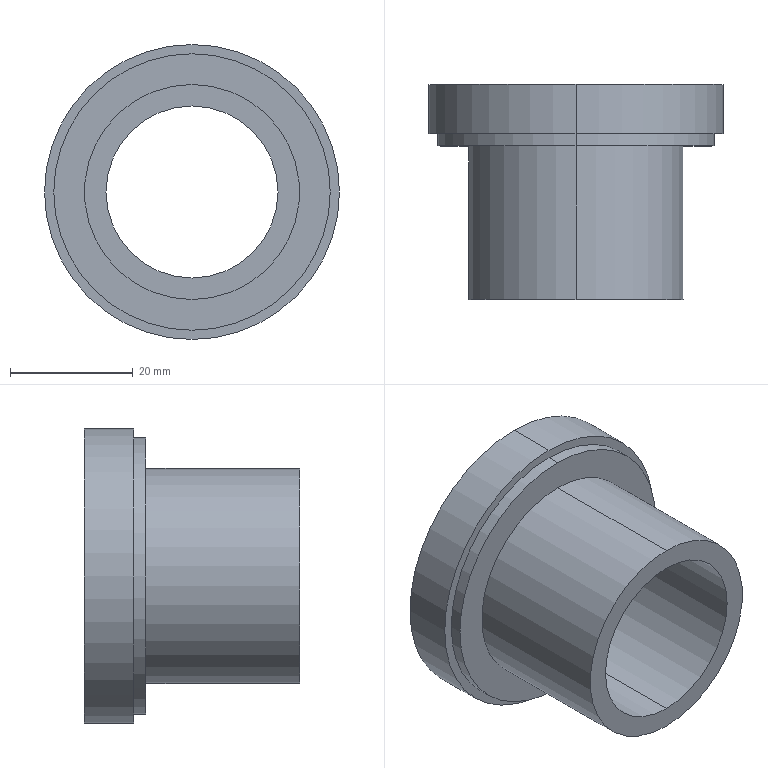Part | SolidWorks | features HoleWzd 1, Revolution 1 | 1 solid | 36 faces | box 48 x 35 x 48 mm | volume 19426 mm3 | cylinder 20 | cone 12 | plane 4 | commonest cylinder face diameters 4.2 x12 28 x2 35 x2 45 x2 48 x2
STEP:
#1=CARTESIAN_POINT('',(-19.,26.6,-2.1));
#2=VERTEX_POINT('',#1);
#3=CARTESIAN_POINT('',(-19.,26.6,2.1));
#4=VERTEX_POINT('',#3);
#5=CARTESIAN_POINT('',(-19.,26.6,0.));
#6=DIRECTION('',(0.,1.,0.));
#7=DIRECTION('',(0.,0.,1.));
#8=AXIS2_PLACEMENT_3D('',#5,#6,#7);
#9=CIRCLE('',#8,2.1);
#10=EDGE_CURVE('',#2,#4,#9,.T.);
#11=ORIENTED_EDGE('',*,*,#10,.F.);
#12=CARTESIAN_POINT('',(-19.,35.,-2.1));
#13=VERTEX_POINT('',#12);
#14=CARTESIAN_POINT('',(-19.,35.,-2.1));
#15=DIRECTION('',(0.,1.,0.));
#16=VECTOR('',#15,1000.);
#17=LINE('',#14,#16);
#18=EDGE_CURVE('',#2,#13,#17,.T.);
#19=ORIENTED_EDGE('',*,*,#18,.T.);
#20=CARTESIAN_POINT('',(-19.,35.,2.1));
#21=VERTEX_POINT('',#20);
#22=CARTESIAN_POINT('',(-19.,35.,0.));
#23=DIRECTION('',(0.,1.,0.));
#24=DIRECTION('',(0.,0.,1.));
#25=AXIS2_PLACEMENT_3D('',#22,#23,#24);
#26=CIRCLE('',#25,2.1);
#27=EDGE_CURVE('',#13,#21,#26,.T.);
#28=ORIENTED_EDGE('',*,*,#27,.T.);
#29=CARTESIAN_POINT('',(-19.,35.,2.1));
#30=DIRECTION('',(0.,1.,0.));
#31=VECTOR('',#30,1000.);
#32=LINE('',#29,#31);
#33=EDGE_CURVE('',#4,#21,#32,.T.);
#34=ORIENTED_EDGE('',*,*,#33,.F.);
#35=EDGE_LOOP('',(#11,#19,#28,#34));
#36=FACE_OUTER_BOUND('',#35,.T.);
#37=CARTESIAN_POINT('',(-19.,35.,0.));
#38=DIRECTION('',(0.,1.,0.));
#39=DIRECTION('',(0.,0.,1.));
#40=AXIS2_PLACEMENT_3D('',#37,#38,#39);
#41=CYLINDRICAL_SURFACE('',#40,2.1);
#42=ADVANCED_FACE('',(#36),#41,.F.);
#43=CARTESIAN_POINT('',(-19.,25.338,0.));
#44=VERTEX_POINT('',#43);
#45=CARTESIAN_POINT('',(-19.,26.6,2.1));
#46=DIRECTION('',(0.,0.515,0.8572));
#47=VECTOR('',#46,1000.);
#48=LINE('',#45,#47);
#49=EDGE_CURVE('',#44,#4,#48,.T.);
#50=ORIENTED_EDGE('',*,*,#49,.F.);
#51=CARTESIAN_POINT('',(-19.,26.6,-2.1));
#52=DIRECTION('',(0.,0.515,-0.8572));
#53=VECTOR('',#52,1000.);
#54=LINE('',#51,#53);
#55=EDGE_CURVE('',#44,#2,#54,.T.);
#56=ORIENTED_EDGE('',*,*,#55,.T.);
#57=ORIENTED_EDGE('',*,*,#10,.T.);
#58=EDGE_LOOP('',(#50,#56,#57));
#59=FACE_OUTER_BOUND('',#58,.T.);
#60=CARTESIAN_POINT('',(-19.,26.6,0.));
#61=DIRECTION('',(0.,1.,0.));
#62=DIRECTION('',(0.,0.,1.));
#63=AXIS2_PLACEMENT_3D('',#60,#61,#62);
#64=CONICAL_SURFACE('',#63,2.1,1.03);
#65=ADVANCED_FACE('',(#59),#64,.F.);
#66=CARTESIAN_POINT('',(19.,26.6,-2.1));
#67=VERTEX_POINT('',#66);
#68=CARTESIAN_POINT('',(19.,26.6,2.1));
#69=VERTEX_POINT('',#68);
#70=CARTESIAN_POINT('',(19.,26.6,0.));
#71=DIRECTION('',(0.,1.,0.));
#72=DIRECTION('',(0.,0.,1.));
#73=AXIS2_PLACEMENT_3D('',#70,#71,#72);
#74=CIRCLE('',#73,2.1);
#75=EDGE_CURVE('',#67,#69,#74,.T.);
#76=ORIENTED_EDGE('',*,*,#75,.F.);
#77=CARTESIAN_POINT('',(19.,35.,-2.1));
#78=VERTEX_POINT('',#77);
#79=CARTESIAN_POINT('',(19.,35.,-2.1));
#80=DIRECTION('',(0.,1.,0.));
#81=VECTOR('',#80,1000.);
#82=LINE('',#79,#81);
#83=EDGE_CURVE('',#67,#78,#82,.T.);
#84=ORIENTED_EDGE('',*,*,#83,.T.);
#85=CARTESIAN_POINT('',(19.,35.,2.1));
#86=VERTEX_POINT('',#85);
#87=CARTESIAN_POINT('',(19.,35.,0.));
#88=DIRECTION('',(0.,1.,0.));
#89=DIRECTION('',(0.,0.,1.));
#90=AXIS2_PLACEMENT_3D('',#87,#88,#89);
#91=CIRCLE('',#90,2.1);
#92=EDGE_CURVE('',#78,#86,#91,.T.);
#93=ORIENTED_EDGE('',*,*,#92,.T.);
#94=CARTESIAN_POINT('',(19.,35.,2.1));
#95=DIRECTION('',(0.,1.,0.));
#96=VECTOR('',#95,1000.);
#97=LINE('',#94,#96);
#98=EDGE_CURVE('',#69,#86,#97,.T.);
#99=ORIENTED_EDGE('',*,*,#98,.F.);
#100=EDGE_LOOP('',(#76,#84,#93,#99));
#101=FACE_OUTER_BOUND('',#100,.T.);
#102=CARTESIAN_POINT('',(19.,35.,0.));
#103=DIRECTION('',(0.,1.,0.));
#104=DIRECTION('',(0.,0.,1.));
#105=AXIS2_PLACEMENT_3D('',#102,#103,#104);
#106=CYLINDRICAL_SURFACE('',#105,2.1);
#107=ADVANCED_FACE('',(#101),#106,.F.);
#108=CARTESIAN_POINT('',(19.,25.338,0.));
#109=VERTEX_POINT('',#108);
#110=CARTESIAN_POINT('',(19.,26.6,2.1));
#111=DIRECTION('',(0.,0.515,0.8572));
#112=VECTOR('',#111,1000.);
#113=LINE('',#110,#112);
#114=EDGE_CURVE('',#109,#69,#113,.T.);
#115=ORIENTED_EDGE('',*,*,#114,.F.);
#116=CARTESIAN_POINT('',(19.,26.6,-2.1));
#117=DIRECTION('',(0.,0.515,-0.8572));
#118=VECTOR('',#117,1000.);
#119=LINE('',#116,#118);
#120=EDGE_CURVE('',#109,#67,#119,.T.);
#121=ORIENTED_EDGE('',*,*,#120,.T.);
#122=ORIENTED_EDGE('',*,*,#75,.T.);
#123=EDGE_LOOP('',(#115,#121,#122));
#124=FACE_OUTER_BOUND('',#123,.T.);
#125=CARTESIAN_POINT('',(19.,26.6,0.));
#126=DIRECTION('',(0.,1.,0.));
#127=DIRECTION('',(0.,0.,1.));
#128=AXIS2_PLACEMENT_3D('',#125,#126,#127);
#129=CONICAL_SURFACE('',#128,2.1,1.03);
#130=ADVANCED_FACE('',(#124),#129,.F.);
#131=CARTESIAN_POINT('',(13.435,26.6,-15.535));
#132=VERTEX_POINT('',#131);
#133=CARTESIAN_POINT('',(13.435,26.6,-11.335));
#134=VERTEX_POINT('',#133);
#135=CARTESIAN_POINT('',(13.435,26.6,-13.435));
#136=DIRECTION('',(0.,1.,0.));
#137=DIRECTION('',(0.,0.,1.));
#138=AXIS2_PLACEMENT_3D('',#135,#136,#137);
#139=CIRCLE('',#138,2.1);
#140=EDGE_CURVE('',#132,#134,#139,.T.);
#141=ORIENTED_EDGE('',*,*,#140,.F.);
#142=CARTESIAN_POINT('',(13.435,35.,-15.535));
#143=VERTEX_POINT('',#142);
#144=CARTESIAN_POINT('',(13.435,35.,-15.535));
#145=DIRECTION('',(0.,1.,0.));
#146=VECTOR('',#145,1000.);
#147=LINE('',#144,#146);
#148=EDGE_CURVE('',#132,#143,#147,.T.);
#149=ORIENTED_EDGE('',*,*,#148,.T.);
#150=CARTESIAN_POINT('',(13.435,35.,-11.335));
#151=VERTEX_POINT('',#150);
#152=CARTESIAN_POINT('',(13.435,35.,-13.435));
#153=DIRECTION('',(0.,1.,0.));
#154=DIRECTION('',(0.,0.,1.));
#155=AXIS2_PLACEMENT_3D('',#152,#153,#154);
#156=CIRCLE('',#155,2.1);
#157=EDGE_CURVE('',#143,#151,#156,.T.);
#158=ORIENTED_EDGE('',*,*,#157,.T.);
#159=CARTESIAN_POINT('',(13.435,35.,-11.335));
#160=DIRECTION('',(0.,1.,0.));
#161=VECTOR('',#160,1000.);
#162=LINE('',#159,#161);
#163=EDGE_CURVE('',#134,#151,#162,.T.);
#164=ORIENTED_EDGE('',*,*,#163,.F.);
#165=EDGE_LOOP('',(#141,#149,#158,#164));
#166=FACE_OUTER_BOUND('',#165,.T.);
#167=CARTESIAN_POINT('',(13.435,35.,-13.435));
#168=DIRECTION('',(0.,1.,0.));
#169=DIRECTION('',(0.,0.,1.));
#170=AXIS2_PLACEMENT_3D('',#167,#168,#169);
#171=CYLINDRICAL_SURFACE('',#170,2.1);
#172=ADVANCED_FACE('',(#166),#171,.F.);
#173=CARTESIAN_POINT('',(13.435,25.338,-13.435));
#174=VERTEX_POINT('',#173);
#175=CARTESIAN_POINT('',(13.435,26.6,-11.335));
#176=DIRECTION('',(0.,0.515,0.8572));
#177=VECTOR('',#176,1000.);
#178=LINE('',#175,#177);
#179=EDGE_CURVE('',#174,#134,#178,.T.);
#180=ORIENTED_EDGE('',*,*,#179,.F.);
#181=CARTESIAN_POINT('',(13.435,26.6,-15.535));
#182=DIRECTION('',(0.,0.515,-0.8572));
#183=VECTOR('',#182,1000.);
#184=LINE('',#181,#183);
#185=EDGE_CURVE('',#174,#132,#184,.T.);
#186=ORIENTED_EDGE('',*,*,#185,.T.);
#187=ORIENTED_EDGE('',*,*,#140,.T.);
#188=EDGE_LOOP('',(#180,#186,#187));
#189=FACE_OUTER_BOUND('',#188,.T.);
#190=CARTESIAN_POINT('',(13.435,26.6,-13.435));
#191=DIRECTION('',(0.,1.,0.));
#192=DIRECTION('',(0.,0.,1.));
#193=AXIS2_PLACEMENT_3D('',#190,#191,#192);
#194=CONICAL_SURFACE('',#193,2.1,1.03);
#195=ADVANCED_FACE('',(#189),#194,.F.);
#196=CARTESIAN_POINT('',(13.435,26.6,11.335));
#197=VERTEX_POINT('',#196);
#198=CARTESIAN_POINT('',(13.435,26.6,15.535));
#199=VERTEX_POINT('',#198);
#200=CARTESIAN_POINT('',(13.435,26.6,13.435));
#201=DIRECTION('',(0.,1.,0.));
#202=DIRECTION('',(0.,0.,1.));
#203=AXIS2_PLACEMENT_3D('',#200,#201,#202);
#204=CIRCLE('',#203,2.1);
#205=EDGE_CURVE('',#197,#199,#204,.T.);
#206=ORIENTED_EDGE('',*,*,#205,.F.);
#207=CARTESIAN_POINT('',(13.435,35.,11.335));
#208=VERTEX_POINT('',#207);
#209=CARTESIAN_POINT('',(13.435,35.,11.335));
#210=DIRECTION('',(0.,1.,0.));
#211=VECTOR('',#210,1000.);
#212=LINE('',#209,#211);
#213=EDGE_CURVE('',#197,#208,#212,.T.);
#214=ORIENTED_EDGE('',*,*,#213,.T.);
#215=CARTESIAN_POINT('',(13.435,35.,15.535));
#216=VERTEX_POINT('',#215);
#217=CARTESIAN_POINT('',(13.435,35.,13.435));
#218=DIRECTION('',(0.,1.,0.));
#219=DIRECTION('',(0.,0.,1.));
#220=AXIS2_PLACEMENT_3D('',#217,#218,#219);
#221=CIRCLE('',#220,2.1);
#222=EDGE_CURVE('',#208,#216,#221,.T.);
#223=ORIENTED_EDGE('',*,*,#222,.T.);
#224=CARTESIAN_POINT('',(13.435,35.,15.535));
#225=DIRECTION('',(0.,1.,0.));
#226=VECTOR('',#225,1000.);
#227=LINE('',#224,#226);
#228=EDGE_CURVE('',#199,#216,#227,.T.);
#229=ORIENTED_EDGE('',*,*,#228,.F.);
#230=EDGE_LOOP('',(#206,#214,#223,#229));
#231=FACE_OUTER_BOUND('',#230,.T.);
#232=CARTESIAN_POINT('',(13.435,35.,13.435));
#233=DIRECTION('',(0.,1.,0.));
#234=DIRECTION('',(0.,0.,1.));
#235=AXIS2_PLACEMENT_3D('',#232,#233,#234);
#236=CYLINDRICAL_SURFACE('',#235,2.1);
#237=ADVANCED_FACE('',(#231),#236,.F.);
#238=CARTESIAN_POINT('',(13.435,25.338,13.435));
#239=VERTEX_POINT('',#238);
#240=CARTESIAN_POINT('',(13.435,26.6,15.535));
#241=DIRECTION('',(0.,0.515,0.8572));
#242=VECTOR('',#241,1000.);
#243=LINE('',#240,#242);
#244=EDGE_CURVE('',#239,#199,#243,.T.);
#245=ORIENTED_EDGE('',*,*,#244,.F.);
#246=CARTESIAN_POINT('',(13.435,26.6,11.335));
#247=DIRECTION('',(0.,0.515,-0.8572));
#248=VECTOR('',#247,1000.);
#249=LINE('',#246,#248);
#250=EDGE_CURVE('',#239,#197,#249,.T.);
#251=ORIENTED_EDGE('',*,*,#250,.T.);
#252=ORIENTED_EDGE('',*,*,#205,.T.);
#253=EDGE_LOOP('',(#245,#251,#252));
#254=FACE_OUTER_BOUND('',#253,.T.);
#255=CARTESIAN_POINT('',(13.435,26.6,13.435));
#256=DIRECTION('',(0.,1.,0.));
#257=DIRECTION('',(0.,0.,1.));
#258=AXIS2_PLACEMENT_3D('',#255,#256,#257);
#259=CONICAL_SURFACE('',#258,2.1,1.03);
#260=ADVANCED_FACE('',(#254),#259,.F.);
#261=CARTESIAN_POINT('',(-13.435,26.6,11.335));
#262=VERTEX_POINT('',#261);
#263=CARTESIAN_POINT('',(-13.435,26.6,15.535));
#264=VERTEX_POINT('',#263);
#265=CARTESIAN_POINT('',(-13.435,26.6,13.435));
#266=DIRECTION('',(0.,1.,0.));
#267=DIRECTION('',(0.,0.,1.));
#268=AXIS2_PLACEMENT_3D('',#265,#266,#267);
#269=CIRCLE('',#268,2.1);
#270=EDGE_CURVE('',#262,#264,#269,.T.);
#271=ORIENTED_EDGE('',*,*,#270,.F.);
#272=CARTESIAN_POINT('',(-13.435,35.,11.335));
#273=VERTEX_POINT('',#272);
#274=CARTESIAN_POINT('',(-13.435,35.,11.335));
#275=DIRECTION('',(0.,1.,0.));
#276=VECTOR('',#275,1000.);
#277=LINE('',#274,#276);
#278=EDGE_CURVE('',#262,#273,#277,.T.);
#279=ORIENTED_EDGE('',*,*,#278,.T.);
#280=CARTESIAN_POINT('',(-13.435,35.,15.535));
#281=VERTEX_POINT('',#280);
#282=CARTESIAN_POINT('',(-13.435,35.,13.435));
#283=DIRECTION('',(0.,1.,0.));
#284=DIRECTION('',(0.,0.,1.));
#285=AXIS2_PLACEMENT_3D('',#282,#283,#284);
#286=CIRCLE('',#285,2.1);
#287=EDGE_CURVE('',#273,#281,#286,.T.);
#288=ORIENTED_EDGE('',*,*,#287,.T.);
#289=CARTESIAN_POINT('',(-13.435,35.,15.535));
#290=DIRECTION('',(0.,1.,0.));
#291=VECTOR('',#290,1000.);
#292=LINE('',#289,#291);
#293=EDGE_CURVE('',#264,#281,#292,.T.);
#294=ORIENTED_EDGE('',*,*,#293,.F.);
#295=EDGE_LOOP('',(#271,#279,#288,#294));
#296=FACE_OUTER_BOUND('',#295,.T.);
#297=CARTESIAN_POINT('',(-13.435,35.,13.435));
#298=DIRECTION('',(0.,1.,0.));
#299=DIRECTION('',(0.,0.,1.));
#300=AXIS2_PLACEMENT_3D('',#297,#298,#299);
#301=CYLINDRICAL_SURFACE('',#300,2.1);
#302=ADVANCED_FACE('',(#296),#301,.F.);
#303=CARTESIAN_POINT('',(-13.435,25.338,13.435));
#304=VERTEX_POINT('',#303);
#305=CARTESIAN_POINT('',(-13.435,26.6,15.535));
#306=DIRECTION('',(0.,0.515,0.8572));
#307=VECTOR('',#306,1000.);
#308=LINE('',#305,#307);
#309=EDGE_CURVE('',#304,#264,#308,.T.);
#310=ORIENTED_EDGE('',*,*,#309,.F.);
#311=CARTESIAN_POINT('',(-13.435,26.6,11.335));
#312=DIRECTION('',(0.,0.515,-0.8572));
#313=VECTOR('',#312,1000.);
#314=LINE('',#311,#313);
#315=EDGE_CURVE('',#304,#262,#314,.T.);
#316=ORIENTED_EDGE('',*,*,#315,.T.);
#317=ORIENTED_EDGE('',*,*,#270,.T.);
#318=EDGE_LOOP('',(#310,#316,#317));
#319=FACE_OUTER_BOUND('',#318,.T.);
#320=CARTESIAN_POINT('',(-13.435,26.6,13.435));
#321=DIRECTION('',(0.,1.,0.));
#322=DIRECTION('',(0.,0.,1.));
#323=AXIS2_PLACEMENT_3D('',#320,#321,#322);
#324=CONICAL_SURFACE('',#323,2.1,1.03);
#325=ADVANCED_FACE('',(#319),#324,.F.);
#326=CARTESIAN_POINT('',(-13.435,26.6,-15.535));
#327=VERTEX_POINT('',#326);
#328=CARTESIAN_POINT('',(-13.435,26.6,-11.335));
#329=VERTEX_POINT('',#328);
#330=CARTESIAN_POINT('',(-13.435,26.6,-13.435));
#331=DIRECTION('',(0.,1.,0.));
#332=DIRECTION('',(0.,0.,1.));
#333=AXIS2_PLACEMENT_3D('',#330,#331,#332);
#334=CIRCLE('',#333,2.1);
#335=EDGE_CURVE('',#327,#329,#334,.T.);
#336=ORIENTED_EDGE('',*,*,#335,.F.);
#337=CARTESIAN_POINT('',(-13.435,35.,-15.535));
#338=VERTEX_POINT('',#337);
#339=CARTESIAN_POINT('',(-13.435,35.,-15.535));
#340=DIRECTION('',(0.,1.,0.));
#341=VECTOR('',#340,1000.);
#342=LINE('',#339,#341);
#343=EDGE_CURVE('',#327,#338,#342,.T.);
#344=ORIENTED_EDGE('',*,*,#343,.T.);
#345=CARTESIAN_POINT('',(-13.435,35.,-11.335));
#346=VERTEX_POINT('',#345);
#347=CARTESIAN_POINT('',(-13.435,35.,-13.435));
#348=DIRECTION('',(0.,1.,0.));
#349=DIRECTION('',(0.,0.,1.));
#350=AXIS2_PLACEMENT_3D('',#347,#348,#349);
#351=CIRCLE('',#350,2.1);
#352=EDGE_CURVE('',#338,#346,#351,.T.);
#353=ORIENTED_EDGE('',*,*,#352,.T.);
#354=CARTESIAN_POINT('',(-13.435,35.,-11.335));
#355=DIRECTION('',(0.,1.,0.));
#356=VECTOR('',#355,1000.);
#357=LINE('',#354,#356);
#358=EDGE_CURVE('',#329,#346,#357,.T.);
#359=ORIENTED_EDGE('',*,*,#358,.F.);
#360=EDGE_LOOP('',(#336,#344,#353,#359));
#361=FACE_OUTER_BOUND('',#360,.T.);
#362=CARTESIAN_POINT('',(-13.435,35.,-13.435));
#363=DIRECTION('',(0.,1.,0.));
#364=DIRECTION('',(0.,0.,1.));
#365=AXIS2_PLACEMENT_3D('',#362,#363,#364);
#366=CYLINDRICAL_SURFACE('',#365,2.1);
#367=ADVANCED_FACE('',(#361),#366,.F.);
#368=CARTESIAN_POINT('',(-13.435,25.338,-13.435));
#369=VERTEX_POINT('',#368);
#370=CARTESIAN_POINT('',(-13.435,26.6,-11.335));
#371=DIRECTION('',(0.,0.515,0.8572));
#372=VECTOR('',#371,1000.);
#373=LINE('',#370,#372);
#374=EDGE_CURVE('',#369,#329,#373,.T.);
#375=ORIENTED_EDGE('',*,*,#374,.F.);
#376=CARTESIAN_POINT('',(-13.435,26.6,-15.535));
#377=DIRECTION('',(0.,0.515,-0.8572));
#378=VECTOR('',#377,1000.);
#379=LINE('',#376,#378);
#380=EDGE_CURVE('',#369,#327,#379,.T.);
#381=ORIENTED_EDGE('',*,*,#380,.T.);
#382=ORIENTED_EDGE('',*,*,#335,.T.);
#383=EDGE_LOOP('',(#375,#381,#382));
#384=FACE_OUTER_BOUND('',#383,.T.);
#385=CARTESIAN_POINT('',(-13.435,26.6,-13.435));
#386=DIRECTION('',(0.,1.,0.));
#387=DIRECTION('',(0.,0.,1.));
#388=AXIS2_PLACEMENT_3D('',#385,#386,#387);
#389=CONICAL_SURFACE('',#388,2.1,1.03);
#390=ADVANCED_FACE('',(#384),#389,.F.);
#391=CARTESIAN_POINT('',(0.,35.,-24.));
#392=VERTEX_POINT('',#391);
#393=CARTESIAN_POINT('',(0.,35.,24.));
#394=VERTEX_POINT('',#393);
#395=CARTESIAN_POINT('',(0.,35.,0.));
#396=DIRECTION('',(0.,-1.,0.));
#397=DIRECTION('',(0.,0.,-1.));
#398=AXIS2_PLACEMENT_3D('',#395,#396,#397);
#399=CIRCLE('',#398,24.);
#400=EDGE_CURVE('',#392,#394,#399,.T.);
#401=ORIENTED_EDGE('',*,*,#400,.T.);
#402=CARTESIAN_POINT('',(0.,27.,24.));
#403=VERTEX_POINT('',#402);
#404=CARTESIAN_POINT('',(0.,0.,24.));
#405=DIRECTION('',(0.,-1.,0.));
#406=VECTOR('',#405,1000.);
#407=LINE('',#404,#406);
#408=EDGE_CURVE('',#394,#403,#407,.T.);
#409=ORIENTED_EDGE('',*,*,#408,.T.);
#410=CARTESIAN_POINT('',(0.,27.,-24.));
#411=VERTEX_POINT('',#410);
#412=CARTESIAN_POINT('',(0.,27.,0.));
#413=DIRECTION('',(0.,-1.,0.));
#414=DIRECTION('',(0.,0.,-1.));
#415=AXIS2_PLACEMENT_3D('',#412,#413,#414);
#416=CIRCLE('',#415,24.);
#417=EDGE_CURVE('',#411,#403,#416,.T.);
#418=ORIENTED_EDGE('',*,*,#417,.F.);
#419=CARTESIAN_POINT('',(0.,0.,-24.));
#420=DIRECTION('',(0.,-1.,0.));
#421=VECTOR('',#420,1000.);
#422=LINE('',#419,#421);
#423=EDGE_CURVE('',#392,#411,#422,.T.);
#424=ORIENTED_EDGE('',*,*,#423,.F.);
#425=EDGE_LOOP('',(#401,#409,#418,#424));
#426=FACE_OUTER_BOUND('',#425,.T.);
#427=CARTESIAN_POINT('',(0.,0.,0.));
#428=DIRECTION('',(0.,-1.,0.));
#429=DIRECTION('',(0.,0.,-1.));
#430=AXIS2_PLACEMENT_3D('',#427,#428,#429);
#431=CYLINDRICAL_SURFACE('',#430,24.);
#432=ADVANCED_FACE('',(#426),#431,.T.);
#433=CARTESIAN_POINT('',(0.,27.,-22.5));
#434=VERTEX_POINT('',#433);
#435=CARTESIAN_POINT('',(0.,27.,22.5));
#436=VERTEX_POINT('',#435);
#437=CARTESIAN_POINT('',(0.,27.,0.));
#438=DIRECTION('',(0.,-1.,0.));
#439=DIRECTION('',(0.,0.,-1.));
#440=AXIS2_PLACEMENT_3D('',#437,#438,#439);
#441=CIRCLE('',#440,22.5);
#442=EDGE_CURVE('',#434,#436,#441,.T.);
#443=ORIENTED_EDGE('',*,*,#442,.T.);
#444=CARTESIAN_POINT('',(0.,25.,22.5));
#445=VERTEX_POINT('',#444);
#446=CARTESIAN_POINT('',(0.,0.,22.5));
#447=DIRECTION('',(0.,-1.,0.));
#448=VECTOR('',#447,1000.);
#449=LINE('',#446,#448);
#450=EDGE_CURVE('',#436,#445,#449,.T.);
#451=ORIENTED_EDGE('',*,*,#450,.T.);
#452=CARTESIAN_POINT('',(0.,25.,-22.5));
#453=VERTEX_POINT('',#452);
#454=CARTESIAN_POINT('',(0.,25.,0.));
#455=DIRECTION('',(0.,-1.,0.));
#456=DIRECTION('',(0.,0.,-1.));
#457=AXIS2_PLACEMENT_3D('',#454,#455,#456);
#458=CIRCLE('',#457,22.5);
#459=EDGE_CURVE('',#453,#445,#458,.T.);
#460=ORIENTED_EDGE('',*,*,#459,.F.);
#461=CARTESIAN_POINT('',(0.,0.,-22.5));
#462=DIRECTION('',(0.,-1.,0.));
#463=VECTOR('',#462,1000.);
#464=LINE('',#461,#463);
#465=EDGE_CURVE('',#434,#453,#464,.T.);
#466=ORIENTED_EDGE('',*,*,#465,.F.);
#467=EDGE_LOOP('',(#443,#451,#460,#466));
#468=FACE_OUTER_BOUND('',#467,.T.);
#469=CARTESIAN_POINT('',(0.,0.,0.));
#470=DIRECTION('',(0.,-1.,0.));
#471=DIRECTION('',(0.,0.,-1.));
#472=AXIS2_PLACEMENT_3D('',#469,#470,#471);
#473=CYLINDRICAL_SURFACE('',#472,22.5);
#474=ADVANCED_FACE('',(#468),#473,.T.);
#475=CARTESIAN_POINT('',(0.,25.,-17.5));
#476=VERTEX_POINT('',#475);
#477=CARTESIAN_POINT('',(0.,25.,17.5));
#478=VERTEX_POINT('',#477);
#479=CARTESIAN_POINT('',(0.,25.,0.));
#480=DIRECTION('',(0.,-1.,0.));
#481=DIRECTION('',(0.,0.,-1.));
#482=AXIS2_PLACEMENT_3D('',#479,#480,#481);
#483=CIRCLE('',#482,17.5);
#484=EDGE_CURVE('',#476,#478,#483,.T.);
#485=ORIENTED_EDGE('',*,*,#484,.T.);
#486=CARTESIAN_POINT('',(0.,0.,17.5));
#487=VERTEX_POINT('',#486);
#488=CARTESIAN_POINT('',(0.,0.,17.5));
#489=DIRECTION('',(0.,-1.,0.));
#490=VECTOR('',#489,1000.);
#491=LINE('',#488,#490);
#492=EDGE_CURVE('',#478,#487,#491,.T.);
#493=ORIENTED_EDGE('',*,*,#492,.T.);
#494=CARTESIAN_POINT('',(0.,0.,-17.5));
#495=VERTEX_POINT('',#494);
#496=CARTESIAN_POINT('',(0.,0.,0.));
#497=DIRECTION('',(0.,-1.,0.));
#498=DIRECTION('',(0.,0.,-1.));
#499=AXIS2_PLACEMENT_3D('',#496,#497,#498);
#500=CIRCLE('',#499,17.5);
#501=EDGE_CURVE('',#495,#487,#500,.T.);
#502=ORIENTED_EDGE('',*,*,#501,.F.);
#503=CARTESIAN_POINT('',(0.,0.,-17.5));
#504=DIRECTION('',(0.,-1.,0.));
#505=VECTOR('',#504,1000.);
#506=LINE('',#503,#505);
#507=EDGE_CURVE('',#476,#495,#506,.T.);
#508=ORIENTED_EDGE('',*,*,#507,.F.);
#509=EDGE_LOOP('',(#485,#493,#502,#508));
#510=FACE_OUTER_BOUND('',#509,.T.);
#511=CARTESIAN_POINT('',(0.,0.,0.));
#512=DIRECTION('',(0.,-1.,0.));
#513=DIRECTION('',(0.,0.,-1.));
#514=AXIS2_PLACEMENT_3D('',#511,#512,#513);
#515=CYLINDRICAL_SURFACE('',#514,17.5);
#516=ADVANCED_FACE('',(#510),#515,.T.);
#517=CARTESIAN_POINT('',(0.,35.,14.));
#518=VERTEX_POINT('',#517);
#519=CARTESIAN_POINT('',(0.,35.,-14.));
#520=VERTEX_POINT('',#519);
#521=CARTESIAN_POINT('',(0.,35.,0.));
#522=DIRECTION('',(0.,-1.,0.));
#523=DIRECTION('',(0.,0.,-1.));
#524=AXIS2_PLACEMENT_3D('',#521,#522,#523);
#525=CIRCLE('',#524,14.);
#526=EDGE_CURVE('',#518,#520,#525,.T.);
#527=ORIENTED_EDGE('',*,*,#526,.F.);
#528=CARTESIAN_POINT('',(0.,0.,14.));
#529=VERTEX_POINT('',#528);
#530=CARTESIAN_POINT('',(0.,0.,14.));
#531=DIRECTION('',(0.,-1.,0.));
#532=VECTOR('',#531,1000.);
#533=LINE('',#530,#532);
#534=EDGE_CURVE('',#518,#529,#533,.T.);
#535=ORIENTED_EDGE('',*,*,#534,.T.);
#536=CARTESIAN_POINT('',(0.,0.,-14.));
#537=VERTEX_POINT('',#536);
#538=CARTESIAN_POINT('',(0.,0.,0.));
#539=DIRECTION('',(0.,-1.,0.));
#540=DIRECTION('',(0.,0.,-1.));
#541=AXIS2_PLACEMENT_3D('',#538,#539,#540);
#542=CIRCLE('',#541,14.);
#543=EDGE_CURVE('',#529,#537,#542,.T.);
#544=ORIENTED_EDGE('',*,*,#543,.T.);
#545=CARTESIAN_POINT('',(0.,0.,-14.));
#546=DIRECTION('',(0.,-1.,0.));
#547=VECTOR('',#546,1000.);
#548=LINE('',#545,#547);
#549=EDGE_CURVE('',#520,#537,#548,.T.);
#550=ORIENTED_EDGE('',*,*,#549,.F.);
#551=EDGE_LOOP('',(#527,#535,#544,#550));
#552=FACE_OUTER_BOUND('',#551,.T.);
#553=CARTESIAN_POINT('',(0.,0.,0.));
#554=DIRECTION('',(0.,-1.,0.));
#555=DIRECTION('',(0.,0.,-1.));
#556=AXIS2_PLACEMENT_3D('',#553,#554,#555);
#557=CYLINDRICAL_SURFACE('',#556,14.);
#558=ADVANCED_FACE('',(#552),#557,.F.);
#559=ORIENTED_EDGE('',*,*,#534,.F.);
#560=CARTESIAN_POINT('',(0.,35.,0.));
#561=DIRECTION('',(0.,-1.,0.));
#562=DIRECTION('',(0.,0.,-1.));
#563=AXIS2_PLACEMENT_3D('',#560,#561,#562);
#564=CIRCLE('',#563,14.);
#565=EDGE_CURVE('',#520,#518,#564,.T.);
#566=ORIENTED_EDGE('',*,*,#565,.F.);
#567=ORIENTED_EDGE('',*,*,#549,.T.);
#568=CARTESIAN_POINT('',(0.,0.,0.));
#569=DIRECTION('',(0.,-1.,0.));
#570=DIRECTION('',(0.,0.,-1.));
#571=AXIS2_PLACEMENT_3D('',#568,#569,#570);
#572=CIRCLE('',#571,14.);
#573=EDGE_CURVE('',#537,#529,#572,.T.);
#574=ORIENTED_EDGE('',*,*,#573,.T.);
#575=EDGE_LOOP('',(#559,#566,#567,#574));
#576=FACE_OUTER_BOUND('',#575,.T.);
#577=CARTESIAN_POINT('',(0.,0.,0.));
#578=DIRECTION('',(0.,-1.,0.));
#579=DIRECTION('',(0.,0.,-1.));
#580=AXIS2_PLACEMENT_3D('',#577,#578,#579);
#581=CYLINDRICAL_SURFACE('',#580,14.);
#582=ADVANCED_FACE('',(#576),#581,.F.);
#583=ORIENTED_EDGE('',*,*,#501,.T.);
#584=CARTESIAN_POINT('',(0.,0.,0.));
#585=DIRECTION('',(0.,-1.,0.));
#586=DIRECTION('',(0.,0.,-1.));
#587=AXIS2_PLACEMENT_3D('',#584,#585,#586);
#588=CIRCLE('',#587,17.5);
#589=EDGE_CURVE('',#487,#495,#588,.T.);
#590=ORIENTED_EDGE('',*,*,#589,.T.);
#591=EDGE_LOOP('',(#583,#590));
#592=FACE_OUTER_BOUND('',#591,.T.);
#593=ORIENTED_EDGE('',*,*,#573,.F.);
#594=ORIENTED_EDGE('',*,*,#543,.F.);
#595=EDGE_LOOP('',(#593,#594));
#596=FACE_BOUND('',#595,.T.);
#597=CARTESIAN_POINT('',(14.,0.,0.));
#598=DIRECTION('',(0.,-1.,0.));
#599=DIRECTION('',(0.,0.,-1.));
#600=AXIS2_PLACEMENT_3D('',#597,#598,#599);
#601=PLANE('',#600);
#602=ADVANCED_FACE('',(#592,#596),#601,.T.);
#603=ORIENTED_EDGE('',*,*,#492,.F.);
#604=CARTESIAN_POINT('',(0.,25.,0.));
#605=DIRECTION('',(0.,-1.,0.));
#606=DIRECTION('',(0.,0.,-1.));
#607=AXIS2_PLACEMENT_3D('',#604,#605,#606);
#608=CIRCLE('',#607,17.5);
#609=EDGE_CURVE('',#478,#476,#608,.T.);
#610=ORIENTED_EDGE('',*,*,#609,.T.);
#611=ORIENTED_EDGE('',*,*,#507,.T.);
#612=ORIENTED_EDGE('',*,*,#589,.F.);
#613=EDGE_LOOP('',(#603,#610,#611,#612));
#614=FACE_OUTER_BOUND('',#613,.T.);
#615=CARTESIAN_POINT('',(0.,0.,0.));
#616=DIRECTION('',(0.,-1.,0.));
#617=DIRECTION('',(0.,0.,-1.));
#618=AXIS2_PLACEMENT_3D('',#615,#616,#617);
#619=CYLINDRICAL_SURFACE('',#618,17.5);
#620=ADVANCED_FACE('',(#614),#619,.T.);
#621=ORIENTED_EDGE('',*,*,#459,.T.);
#622=CARTESIAN_POINT('',(0.,25.,0.));
#623=DIRECTION('',(0.,-1.,0.));
#624=DIRECTION('',(0.,0.,-1.));
#625=AXIS2_PLACEMENT_3D('',#622,#623,#624);
#626=CIRCLE('',#625,22.5);
#627=EDGE_CURVE('',#445,#453,#626,.T.);
#628=ORIENTED_EDGE('',*,*,#627,.T.);
#629=EDGE_LOOP('',(#621,#628));
#630=FACE_OUTER_BOUND('',#629,.T.);
#631=ORIENTED_EDGE('',*,*,#484,.F.);
#632=ORIENTED_EDGE('',*,*,#609,.F.);
#633=EDGE_LOOP('',(#631,#632));
#634=FACE_BOUND('',#633,.T.);
#635=CARTESIAN_POINT('',(17.5,25.,0.));
#636=DIRECTION('',(0.,-1.,0.));
#637=DIRECTION('',(0.,0.,-1.));
#638=AXIS2_PLACEMENT_3D('',#635,#636,#637);
#639=PLANE('',#638);
#640=ADVANCED_FACE('',(#630,#634),#639,.T.);
#641=ORIENTED_EDGE('',*,*,#450,.F.);
#642=CARTESIAN_POINT('',(0.,27.,0.));
#643=DIRECTION('',(0.,-1.,0.));
#644=DIRECTION('',(0.,0.,-1.));
#645=AXIS2_PLACEMENT_3D('',#642,#643,#644);
#646=CIRCLE('',#645,22.5);
#647=EDGE_CURVE('',#436,#434,#646,.T.);
#648=ORIENTED_EDGE('',*,*,#647,.T.);
#649=ORIENTED_EDGE('',*,*,#465,.T.);
#650=ORIENTED_EDGE('',*,*,#627,.F.);
#651=EDGE_LOOP('',(#641,#648,#649,#650));
#652=FACE_OUTER_BOUND('',#651,.T.);
#653=CARTESIAN_POINT('',(0.,0.,0.));
#654=DIRECTION('',(0.,-1.,0.));
#655=DIRECTION('',(0.,0.,-1.));
#656=AXIS2_PLACEMENT_3D('',#653,#654,#655);
#657=CYLINDRICAL_SURFACE('',#656,22.5);
#658=ADVANCED_FACE('',(#652),#657,.T.);
#659=ORIENTED_EDGE('',*,*,#417,.T.);
#660=CARTESIAN_POINT('',(0.,27.,0.));
#661=DIRECTION('',(0.,-1.,0.));
#662=DIRECTION('',(0.,0.,-1.));
#663=AXIS2_PLACEMENT_3D('',#660,#661,#662);
#664=CIRCLE('',#663,24.);
#665=EDGE_CURVE('',#403,#411,#664,.T.);
#666=ORIENTED_EDGE('',*,*,#665,.T.);
#667=EDGE_LOOP('',(#659,#666));
#668=FACE_OUTER_BOUND('',#667,.T.);
#669=ORIENTED_EDGE('',*,*,#442,.F.);
#670=ORIENTED_EDGE('',*,*,#647,.F.);
#671=EDGE_LOOP('',(#669,#670));
#672=FACE_BOUND('',#671,.T.);
#673=CARTESIAN_POINT('',(24.,27.,0.));
#674=DIRECTION('',(0.,-1.,0.));
#675=DIRECTION('',(0.,0.,-1.));
#676=AXIS2_PLACEMENT_3D('',#673,#674,#675);
#677=PLANE('',#676);
#678=ADVANCED_FACE('',(#668,#672),#677,.T.);
#679=ORIENTED_EDGE('',*,*,#408,.F.);
#680=CARTESIAN_POINT('',(0.,35.,0.));
#681=DIRECTION('',(0.,-1.,0.));
#682=DIRECTION('',(0.,0.,-1.));
#683=AXIS2_PLACEMENT_3D('',#680,#681,#682);
#684=CIRCLE('',#683,24.);
#685=EDGE_CURVE('',#394,#392,#684,.T.);
#686=ORIENTED_EDGE('',*,*,#685,.T.);
#687=ORIENTED_EDGE('',*,*,#423,.T.);
#688=ORIENTED_EDGE('',*,*,#665,.F.);
#689=EDGE_LOOP('',(#679,#686,#687,#688));
#690=FACE_OUTER_BOUND('',#689,.T.);
#691=CARTESIAN_POINT('',(0.,0.,0.));
#692=DIRECTION('',(0.,-1.,0.));
#693=DIRECTION('',(0.,0.,-1.));
#694=AXIS2_PLACEMENT_3D('',#691,#692,#693);
#695=CYLINDRICAL_SURFACE('',#694,24.);
#696=ADVANCED_FACE('',(#690),#695,.T.);
#697=CARTESIAN_POINT('',(-19.,35.,0.));
#698=DIRECTION('',(0.,1.,0.));
#699=DIRECTION('',(0.,0.,1.));
#700=AXIS2_PLACEMENT_3D('',#697,#698,#699);
#701=CIRCLE('',#700,2.1);
#702=EDGE_CURVE('',#21,#13,#701,.T.);
#703=ORIENTED_EDGE('',*,*,#702,.F.);
#704=ORIENTED_EDGE('',*,*,#27,.F.);
#705=EDGE_LOOP('',(#703,#704));
#706=FACE_BOUND('',#705,.T.);
#707=CARTESIAN_POINT('',(19.,35.,0.));
#708=DIRECTION('',(0.,1.,0.));
#709=DIRECTION('',(0.,0.,1.));
#710=AXIS2_PLACEMENT_3D('',#707,#708,#709);
#711=CIRCLE('',#710,2.1);
#712=EDGE_CURVE('',#86,#78,#711,.T.);
#713=ORIENTED_EDGE('',*,*,#712,.F.);
#714=ORIENTED_EDGE('',*,*,#92,.F.);
#715=EDGE_LOOP('',(#713,#714));
#716=FACE_BOUND('',#715,.T.);
#717=CARTESIAN_POINT('',(13.435,35.,-13.435));
#718=DIRECTION('',(0.,1.,0.));
#719=DIRECTION('',(0.,0.,1.));
#720=AXIS2_PLACEMENT_3D('',#717,#718,#719);
#721=CIRCLE('',#720,2.1);
#722=EDGE_CURVE('',#151,#143,#721,.T.);
#723=ORIENTED_EDGE('',*,*,#722,.F.);
#724=ORIENTED_EDGE('',*,*,#157,.F.);
#725=EDGE_LOOP('',(#723,#724));
#726=FACE_BOUND('',#725,.T.);
#727=CARTESIAN_POINT('',(13.435,35.,13.435));
#728=DIRECTION('',(0.,1.,0.));
#729=DIRECTION('',(0.,0.,1.));
#730=AXIS2_PLACEMENT_3D('',#727,#728,#729);
#731=CIRCLE('',#730,2.1);
#732=EDGE_CURVE('',#216,#208,#731,.T.);
#733=ORIENTED_EDGE('',*,*,#732,.F.);
#734=ORIENTED_EDGE('',*,*,#222,.F.);
#735=EDGE_LOOP('',(#733,#734));
#736=FACE_BOUND('',#735,.T.);
#737=CARTESIAN_POINT('',(-13.435,35.,13.435));
#738=DIRECTION('',(0.,1.,0.));
#739=DIRECTION('',(0.,0.,1.));
#740=AXIS2_PLACEMENT_3D('',#737,#738,#739);
#741=CIRCLE('',#740,2.1);
#742=EDGE_CURVE('',#281,#273,#741,.T.);
#743=ORIENTED_EDGE('',*,*,#742,.F.);
#744=ORIENTED_EDGE('',*,*,#287,.F.);
#745=EDGE_LOOP('',(#743,#744));
#746=FACE_BOUND('',#745,.T.);
#747=CARTESIAN_POINT('',(-13.435,35.,-13.435));
#748=DIRECTION('',(0.,1.,0.));
#749=DIRECTION('',(0.,0.,1.));
#750=AXIS2_PLACEMENT_3D('',#747,#748,#749);
#751=CIRCLE('',#750,2.1);
#752=EDGE_CURVE('',#346,#338,#751,.T.);
#753=ORIENTED_EDGE('',*,*,#752,.F.);
#754=ORIENTED_EDGE('',*,*,#352,.F.);
#755=EDGE_LOOP('',(#753,#754));
#756=FACE_BOUND('',#755,.T.);
#757=ORIENTED_EDGE('',*,*,#565,.T.);
#758=ORIENTED_EDGE('',*,*,#526,.T.);
#759=EDGE_LOOP('',(#757,#758));
#760=FACE_BOUND('',#759,.T.);
#761=ORIENTED_EDGE('',*,*,#400,.F.);
#762=ORIENTED_EDGE('',*,*,#685,.F.);
#763=EDGE_LOOP('',(#761,#762));
#764=FACE_OUTER_BOUND('',#763,.T.);
#765=CARTESIAN_POINT('',(24.,35.,0.));
#766=DIRECTION('',(0.,1.,0.));
#767=DIRECTION('',(0.,0.,1.));
#768=AXIS2_PLACEMENT_3D('',#765,#766,#767);
#769=PLANE('',#768);
#770=ADVANCED_FACE('',(#706,#716,#726,#736,#746,#756,#760,#764),#769,.T.);
#771=ORIENTED_EDGE('',*,*,#380,.F.);
#772=ORIENTED_EDGE('',*,*,#374,.T.);
#773=CARTESIAN_POINT('',(-13.435,26.6,-13.435));
#774=DIRECTION('',(0.,1.,0.));
#775=DIRECTION('',(0.,0.,1.));
#776=AXIS2_PLACEMENT_3D('',#773,#774,#775);
#777=CIRCLE('',#776,2.1);
#778=EDGE_CURVE('',#329,#327,#777,.T.);
#779=ORIENTED_EDGE('',*,*,#778,.T.);
#780=EDGE_LOOP('',(#771,#772,#779));
#781=FACE_OUTER_BOUND('',#780,.T.);
#782=CARTESIAN_POINT('',(-13.435,26.6,-13.435));
#783=DIRECTION('',(0.,1.,0.));
#784=DIRECTION('',(0.,0.,1.));
#785=AXIS2_PLACEMENT_3D('',#782,#783,#784);
#786=CONICAL_SURFACE('',#785,2.1,1.03);
#787=ADVANCED_FACE('',(#781),#786,.F.);
#788=ORIENTED_EDGE('',*,*,#343,.F.);
#789=ORIENTED_EDGE('',*,*,#778,.F.);
#790=ORIENTED_EDGE('',*,*,#358,.T.);
#791=ORIENTED_EDGE('',*,*,#752,.T.);
#792=EDGE_LOOP('',(#788,#789,#790,#791));
#793=FACE_OUTER_BOUND('',#792,.T.);
#794=CARTESIAN_POINT('',(-13.435,35.,-13.435));
#795=DIRECTION('',(0.,1.,0.));
#796=DIRECTION('',(0.,0.,1.));
#797=AXIS2_PLACEMENT_3D('',#794,#795,#796);
#798=CYLINDRICAL_SURFACE('',#797,2.1);
#799=ADVANCED_FACE('',(#793),#798,.F.);
#800=ORIENTED_EDGE('',*,*,#315,.F.);
#801=ORIENTED_EDGE('',*,*,#309,.T.);
#802=CARTESIAN_POINT('',(-13.435,26.6,13.435));
#803=DIRECTION('',(0.,1.,0.));
#804=DIRECTION('',(0.,0.,1.));
#805=AXIS2_PLACEMENT_3D('',#802,#803,#804);
#806=CIRCLE('',#805,2.1);
#807=EDGE_CURVE('',#264,#262,#806,.T.);
#808=ORIENTED_EDGE('',*,*,#807,.T.);
#809=EDGE_LOOP('',(#800,#801,#808));
#810=FACE_OUTER_BOUND('',#809,.T.);
#811=CARTESIAN_POINT('',(-13.435,26.6,13.435));
#812=DIRECTION('',(0.,1.,0.));
#813=DIRECTION('',(0.,0.,1.));
#814=AXIS2_PLACEMENT_3D('',#811,#812,#813);
#815=CONICAL_SURFACE('',#814,2.1,1.03);
#816=ADVANCED_FACE('',(#810),#815,.F.);
#817=ORIENTED_EDGE('',*,*,#278,.F.);
#818=ORIENTED_EDGE('',*,*,#807,.F.);
#819=ORIENTED_EDGE('',*,*,#293,.T.);
#820=ORIENTED_EDGE('',*,*,#742,.T.);
#821=EDGE_LOOP('',(#817,#818,#819,#820));
#822=FACE_OUTER_BOUND('',#821,.T.);
#823=CARTESIAN_POINT('',(-13.435,35.,13.435));
#824=DIRECTION('',(0.,1.,0.));
#825=DIRECTION('',(0.,0.,1.));
#826=AXIS2_PLACEMENT_3D('',#823,#824,#825);
#827=CYLINDRICAL_SURFACE('',#826,2.1);
#828=ADVANCED_FACE('',(#822),#827,.F.);
#829=ORIENTED_EDGE('',*,*,#250,.F.);
#830=ORIENTED_EDGE('',*,*,#244,.T.);
#831=CARTESIAN_POINT('',(13.435,26.6,13.435));
#832=DIRECTION('',(0.,1.,0.));
#833=DIRECTION('',(0.,0.,1.));
#834=AXIS2_PLACEMENT_3D('',#831,#832,#833);
#835=CIRCLE('',#834,2.1);
#836=EDGE_CURVE('',#199,#197,#835,.T.);
#837=ORIENTED_EDGE('',*,*,#836,.T.);
#838=EDGE_LOOP('',(#829,#830,#837));
#839=FACE_OUTER_BOUND('',#838,.T.);
#840=CARTESIAN_POINT('',(13.435,26.6,13.435));
#841=DIRECTION('',(0.,1.,0.));
#842=DIRECTION('',(0.,0.,1.));
#843=AXIS2_PLACEMENT_3D('',#840,#841,#842);
#844=CONICAL_SURFACE('',#843,2.1,1.03);
#845=ADVANCED_FACE('',(#839),#844,.F.);
#846=ORIENTED_EDGE('',*,*,#213,.F.);
#847=ORIENTED_EDGE('',*,*,#836,.F.);
#848=ORIENTED_EDGE('',*,*,#228,.T.);
#849=ORIENTED_EDGE('',*,*,#732,.T.);
#850=EDGE_LOOP('',(#846,#847,#848,#849));
#851=FACE_OUTER_BOUND('',#850,.T.);
#852=CARTESIAN_POINT('',(13.435,35.,13.435));
#853=DIRECTION('',(0.,1.,0.));
#854=DIRECTION('',(0.,0.,1.));
#855=AXIS2_PLACEMENT_3D('',#852,#853,#854);
#856=CYLINDRICAL_SURFACE('',#855,2.1);
#857=ADVANCED_FACE('',(#851),#856,.F.);
#858=ORIENTED_EDGE('',*,*,#185,.F.);
#859=ORIENTED_EDGE('',*,*,#179,.T.);
#860=CARTESIAN_POINT('',(13.435,26.6,-13.435));
#861=DIRECTION('',(0.,1.,0.));
#862=DIRECTION('',(0.,0.,1.));
#863=AXIS2_PLACEMENT_3D('',#860,#861,#862);
#864=CIRCLE('',#863,2.1);
#865=EDGE_CURVE('',#134,#132,#864,.T.);
#866=ORIENTED_EDGE('',*,*,#865,.T.);
#867=EDGE_LOOP('',(#858,#859,#866));
#868=FACE_OUTER_BOUND('',#867,.T.);
#869=CARTESIAN_POINT('',(13.435,26.6,-13.435));
#870=DIRECTION('',(0.,1.,0.));
#871=DIRECTION('',(0.,0.,1.));
#872=AXIS2_PLACEMENT_3D('',#869,#870,#871);
#873=CONICAL_SURFACE('',#872,2.1,1.03);
#874=ADVANCED_FACE('',(#868),#873,.F.);
#875=ORIENTED_EDGE('',*,*,#148,.F.);
#876=ORIENTED_EDGE('',*,*,#865,.F.);
#877=ORIENTED_EDGE('',*,*,#163,.T.);
#878=ORIENTED_EDGE('',*,*,#722,.T.);
#879=EDGE_LOOP('',(#875,#876,#877,#878));
#880=FACE_OUTER_BOUND('',#879,.T.);
#881=CARTESIAN_POINT('',(13.435,35.,-13.435));
#882=DIRECTION('',(0.,1.,0.));
#883=DIRECTION('',(0.,0.,1.));
#884=AXIS2_PLACEMENT_3D('',#881,#882,#883);
#885=CYLINDRICAL_SURFACE('',#884,2.1);
#886=ADVANCED_FACE('',(#880),#885,.F.);
#887=ORIENTED_EDGE('',*,*,#120,.F.);
#888=ORIENTED_EDGE('',*,*,#114,.T.);
#889=CARTESIAN_POINT('',(19.,26.6,0.));
#890=DIRECTION('',(0.,1.,0.));
#891=DIRECTION('',(0.,0.,1.));
#892=AXIS2_PLACEMENT_3D('',#889,#890,#891);
#893=CIRCLE('',#892,2.1);
#894=EDGE_CURVE('',#69,#67,#893,.T.);
#895=ORIENTED_EDGE('',*,*,#894,.T.);
#896=EDGE_LOOP('',(#887,#888,#895));
#897=FACE_OUTER_BOUND('',#896,.T.);
#898=CARTESIAN_POINT('',(19.,26.6,0.));
#899=DIRECTION('',(0.,1.,0.));
#900=DIRECTION('',(0.,0.,1.));
#901=AXIS2_PLACEMENT_3D('',#898,#899,#900);
#902=CONICAL_SURFACE('',#901,2.1,1.03);
#903=ADVANCED_FACE('',(#897),#902,.F.);
#904=ORIENTED_EDGE('',*,*,#83,.F.);
#905=ORIENTED_EDGE('',*,*,#894,.F.);
#906=ORIENTED_EDGE('',*,*,#98,.T.);
#907=ORIENTED_EDGE('',*,*,#712,.T.);
#908=EDGE_LOOP('',(#904,#905,#906,#907));
#909=FACE_OUTER_BOUND('',#908,.T.);
#910=CARTESIAN_POINT('',(19.,35.,0.));
#911=DIRECTION('',(0.,1.,0.));
#912=DIRECTION('',(0.,0.,1.));
#913=AXIS2_PLACEMENT_3D('',#910,#911,#912);
#914=CYLINDRICAL_SURFACE('',#913,2.1);
#915=ADVANCED_FACE('',(#909),#914,.F.);
#916=ORIENTED_EDGE('',*,*,#55,.F.);
#917=ORIENTED_EDGE('',*,*,#49,.T.);
#918=CARTESIAN_POINT('',(-19.,26.6,0.));
#919=DIRECTION('',(0.,1.,0.));
#920=DIRECTION('',(0.,0.,1.));
#921=AXIS2_PLACEMENT_3D('',#918,#919,#920);
#922=CIRCLE('',#921,2.1);
#923=EDGE_CURVE('',#4,#2,#922,.T.);
#924=ORIENTED_EDGE('',*,*,#923,.T.);
#925=EDGE_LOOP('',(#916,#917,#924));
#926=FACE_OUTER_BOUND('',#925,.T.);
#927=CARTESIAN_POINT('',(-19.,26.6,0.));
#928=DIRECTION('',(0.,1.,0.));
#929=DIRECTION('',(0.,0.,1.));
#930=AXIS2_PLACEMENT_3D('',#927,#928,#929);
#931=CONICAL_SURFACE('',#930,2.1,1.03);
#932=ADVANCED_FACE('',(#926),#931,.F.);
#933=ORIENTED_EDGE('',*,*,#18,.F.);
#934=ORIENTED_EDGE('',*,*,#923,.F.);
#935=ORIENTED_EDGE('',*,*,#33,.T.);
#936=ORIENTED_EDGE('',*,*,#702,.T.);
#937=EDGE_LOOP('',(#933,#934,#935,#936));
#938=FACE_OUTER_BOUND('',#937,.T.);
#939=CARTESIAN_POINT('',(-19.,35.,0.));
#940=DIRECTION('',(0.,1.,0.));
#941=DIRECTION('',(0.,0.,1.));
#942=AXIS2_PLACEMENT_3D('',#939,#940,#941);
#943=CYLINDRICAL_SURFACE('',#942,2.1);
#944=ADVANCED_FACE('',(#938),#943,.F.);
#945=CLOSED_SHELL('',(#42,#65,#107,#130,#172,#195,#237,#260,#302,#325,#367,#390,#432,#474,#516,#558,#582,#602,#620,#640,#658,#678,#696,#770,#787,#799,#816,#828,#845,#857,#874,#886,#903,#915,#932,#944));
#946=MANIFOLD_SOLID_BREP('',#945);
#947=CARTESIAN_POINT('',(0.,0.,0.));
#948=DIRECTION('',(0.,0.,1.));
#949=DIRECTION('',(1.,0.,0.));
#950=AXIS2_PLACEMENT_3D('',#947,#948,#949);
#951=(LENGTH_UNIT()NAMED_UNIT(*)SI_UNIT(.MILLI.,.METRE.));
#952=UNCERTAINTY_MEASURE_WITH_UNIT(LENGTH_MEASURE(0.00001),#951,'','');
#953=(NAMED_UNIT(*)PLANE_ANGLE_UNIT()SI_UNIT($,.RADIAN.));
#954=(NAMED_UNIT(*)SI_UNIT($,.STERADIAN.)SOLID_ANGLE_UNIT());
#955=(GEOMETRIC_REPRESENTATION_CONTEXT(3)GLOBAL_UNCERTAINTY_ASSIGNED_CONTEXT((#952))GLOBAL_UNIT_ASSIGNED_CONTEXT((#951,#953,#954))REPRESENTATION_CONTEXT('',''));
#956=ADVANCED_BREP_SHAPE_REPRESENTATION('',(#946,#950),#955);